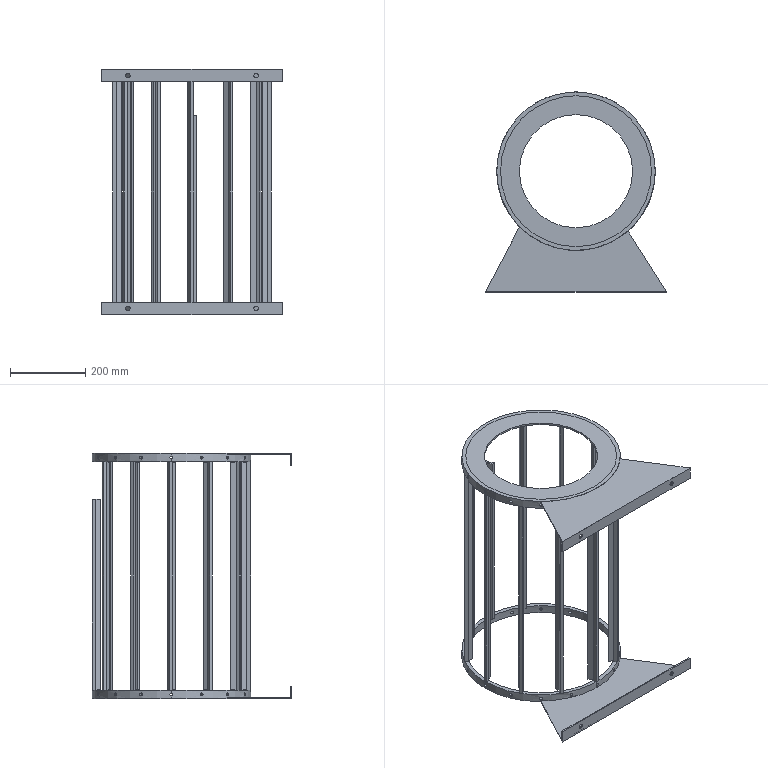Part | SolidWorks | features ICE 8, CirPattern 2, MirrorSolid 2, Extrusion 1 | 29 solids | 250 faces | box 479.111 x 529 x 650 mm | volume 2552099 mm3 | plane 140 | cylinder 110 | commonest cylinder face diameters 8 x64 400 x18 420 x18 12 x8 300 x2